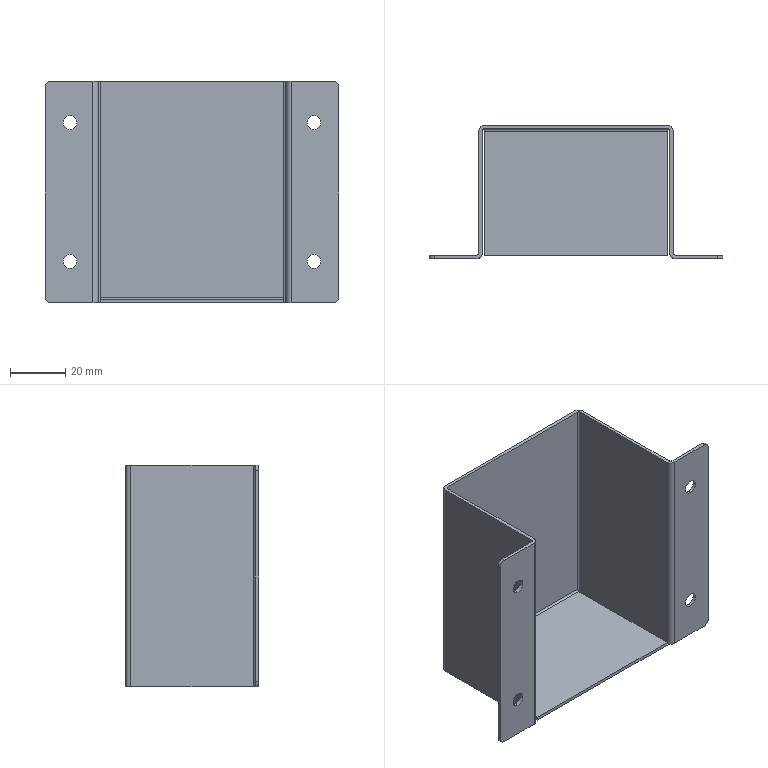Part | SolidWorks | features BaseBody 1 | 1 solid | 44 faces | box 106 x 48 x 80 mm | volume 22432 mm3 | cylinder 22 | plane 22 | commonest cylinder face diameters 5 x8 1.473 x5 3.873 x5 4 x4
STEP:
#1=CARTESIAN_POINT('',(79.,-1.2,67.5));
#2=VERTEX_POINT('',#1);
#3=CARTESIAN_POINT('',(79.,-1.2,62.5));
#4=VERTEX_POINT('',#3);
#5=CARTESIAN_POINT('',(79.,-1.2,65.));
#6=DIRECTION('',(0.,-1.,0.));
#7=DIRECTION('',(0.,0.,1.));
#8=AXIS2_PLACEMENT_3D('',#5,#6,#7);
#9=CIRCLE('',#8,2.5);
#10=EDGE_CURVE('',#2,#4,#9,.T.);
#11=ORIENTED_EDGE('',*,*,#10,.T.);
#12=CARTESIAN_POINT('',(79.,0.,62.5));
#13=VERTEX_POINT('',#12);
#14=CARTESIAN_POINT('',(79.,0.,62.5));
#15=DIRECTION('',(0.,1.,0.));
#16=VECTOR('',#15,1000.);
#17=LINE('',#14,#16);
#18=EDGE_CURVE('',#4,#13,#17,.T.);
#19=ORIENTED_EDGE('',*,*,#18,.T.);
#20=CARTESIAN_POINT('',(79.,0.,67.5));
#21=VERTEX_POINT('',#20);
#22=CARTESIAN_POINT('',(79.,0.,65.));
#23=DIRECTION('',(0.,-1.,0.));
#24=DIRECTION('',(0.,0.,1.));
#25=AXIS2_PLACEMENT_3D('',#22,#23,#24);
#26=CIRCLE('',#25,2.5);
#27=EDGE_CURVE('',#21,#13,#26,.T.);
#28=ORIENTED_EDGE('',*,*,#27,.F.);
#29=CARTESIAN_POINT('',(79.,0.,67.5));
#30=DIRECTION('',(0.,1.,0.));
#31=VECTOR('',#30,1000.);
#32=LINE('',#29,#31);
#33=EDGE_CURVE('',#2,#21,#32,.T.);
#34=ORIENTED_EDGE('',*,*,#33,.F.);
#35=EDGE_LOOP('',(#11,#19,#28,#34));
#36=FACE_OUTER_BOUND('',#35,.T.);
#37=CARTESIAN_POINT('',(79.,0.,65.));
#38=DIRECTION('',(0.,1.,0.));
#39=DIRECTION('',(0.,0.,1.));
#40=AXIS2_PLACEMENT_3D('',#37,#38,#39);
#41=CYLINDRICAL_SURFACE('',#40,2.5);
#42=ADVANCED_FACE('',(#36),#41,.F.);
#43=CARTESIAN_POINT('',(79.,-1.2,17.5));
#44=VERTEX_POINT('',#43);
#45=CARTESIAN_POINT('',(79.,-1.2,12.5));
#46=VERTEX_POINT('',#45);
#47=CARTESIAN_POINT('',(79.,-1.2,15.));
#48=DIRECTION('',(0.,-1.,0.));
#49=DIRECTION('',(0.,0.,1.));
#50=AXIS2_PLACEMENT_3D('',#47,#48,#49);
#51=CIRCLE('',#50,2.5);
#52=EDGE_CURVE('',#44,#46,#51,.T.);
#53=ORIENTED_EDGE('',*,*,#52,.T.);
#54=CARTESIAN_POINT('',(79.,0.,12.5));
#55=VERTEX_POINT('',#54);
#56=CARTESIAN_POINT('',(79.,0.,12.5));
#57=DIRECTION('',(0.,1.,0.));
#58=VECTOR('',#57,1000.);
#59=LINE('',#56,#58);
#60=EDGE_CURVE('',#46,#55,#59,.T.);
#61=ORIENTED_EDGE('',*,*,#60,.T.);
#62=CARTESIAN_POINT('',(79.,0.,17.5));
#63=VERTEX_POINT('',#62);
#64=CARTESIAN_POINT('',(79.,0.,15.));
#65=DIRECTION('',(0.,-1.,0.));
#66=DIRECTION('',(0.,0.,1.));
#67=AXIS2_PLACEMENT_3D('',#64,#65,#66);
#68=CIRCLE('',#67,2.5);
#69=EDGE_CURVE('',#63,#55,#68,.T.);
#70=ORIENTED_EDGE('',*,*,#69,.F.);
#71=CARTESIAN_POINT('',(79.,0.,17.5));
#72=DIRECTION('',(0.,1.,0.));
#73=VECTOR('',#72,1000.);
#74=LINE('',#71,#73);
#75=EDGE_CURVE('',#44,#63,#74,.T.);
#76=ORIENTED_EDGE('',*,*,#75,.F.);
#77=EDGE_LOOP('',(#53,#61,#70,#76));
#78=FACE_OUTER_BOUND('',#77,.T.);
#79=CARTESIAN_POINT('',(79.,0.,15.));
#80=DIRECTION('',(0.,1.,0.));
#81=DIRECTION('',(0.,0.,1.));
#82=AXIS2_PLACEMENT_3D('',#79,#80,#81);
#83=CYLINDRICAL_SURFACE('',#82,2.5);
#84=ADVANCED_FACE('',(#78),#83,.F.);
#85=CARTESIAN_POINT('',(-9.,-1.2,67.5));
#86=VERTEX_POINT('',#85);
#87=CARTESIAN_POINT('',(-9.,-1.2,62.5));
#88=VERTEX_POINT('',#87);
#89=CARTESIAN_POINT('',(-9.,-1.2,65.));
#90=DIRECTION('',(0.,-1.,0.));
#91=DIRECTION('',(0.,0.,1.));
#92=AXIS2_PLACEMENT_3D('',#89,#90,#91);
#93=CIRCLE('',#92,2.5);
#94=EDGE_CURVE('',#86,#88,#93,.T.);
#95=ORIENTED_EDGE('',*,*,#94,.T.);
#96=CARTESIAN_POINT('',(-9.,0.,62.5));
#97=VERTEX_POINT('',#96);
#98=CARTESIAN_POINT('',(-9.,0.,62.5));
#99=DIRECTION('',(0.,1.,0.));
#100=VECTOR('',#99,1000.);
#101=LINE('',#98,#100);
#102=EDGE_CURVE('',#88,#97,#101,.T.);
#103=ORIENTED_EDGE('',*,*,#102,.T.);
#104=CARTESIAN_POINT('',(-9.,0.,67.5));
#105=VERTEX_POINT('',#104);
#106=CARTESIAN_POINT('',(-9.,0.,65.));
#107=DIRECTION('',(0.,-1.,0.));
#108=DIRECTION('',(0.,0.,1.));
#109=AXIS2_PLACEMENT_3D('',#106,#107,#108);
#110=CIRCLE('',#109,2.5);
#111=EDGE_CURVE('',#105,#97,#110,.T.);
#112=ORIENTED_EDGE('',*,*,#111,.F.);
#113=CARTESIAN_POINT('',(-9.,0.,67.5));
#114=DIRECTION('',(0.,1.,0.));
#115=VECTOR('',#114,1000.);
#116=LINE('',#113,#115);
#117=EDGE_CURVE('',#86,#105,#116,.T.);
#118=ORIENTED_EDGE('',*,*,#117,.F.);
#119=EDGE_LOOP('',(#95,#103,#112,#118));
#120=FACE_OUTER_BOUND('',#119,.T.);
#121=CARTESIAN_POINT('',(-9.,0.,65.));
#122=DIRECTION('',(0.,1.,0.));
#123=DIRECTION('',(0.,0.,1.));
#124=AXIS2_PLACEMENT_3D('',#121,#122,#123);
#125=CYLINDRICAL_SURFACE('',#124,2.5);
#126=ADVANCED_FACE('',(#120),#125,.F.);
#127=CARTESIAN_POINT('',(-9.,-1.2,17.5));
#128=VERTEX_POINT('',#127);
#129=CARTESIAN_POINT('',(-9.,-1.2,12.5));
#130=VERTEX_POINT('',#129);
#131=CARTESIAN_POINT('',(-9.,-1.2,15.));
#132=DIRECTION('',(0.,-1.,0.));
#133=DIRECTION('',(0.,0.,1.));
#134=AXIS2_PLACEMENT_3D('',#131,#132,#133);
#135=CIRCLE('',#134,2.5);
#136=EDGE_CURVE('',#128,#130,#135,.T.);
#137=ORIENTED_EDGE('',*,*,#136,.T.);
#138=CARTESIAN_POINT('',(-9.,0.,12.5));
#139=VERTEX_POINT('',#138);
#140=CARTESIAN_POINT('',(-9.,0.,12.5));
#141=DIRECTION('',(0.,1.,0.));
#142=VECTOR('',#141,1000.);
#143=LINE('',#140,#142);
#144=EDGE_CURVE('',#130,#139,#143,.T.);
#145=ORIENTED_EDGE('',*,*,#144,.T.);
#146=CARTESIAN_POINT('',(-9.,0.,17.5));
#147=VERTEX_POINT('',#146);
#148=CARTESIAN_POINT('',(-9.,0.,15.));
#149=DIRECTION('',(0.,-1.,0.));
#150=DIRECTION('',(0.,0.,1.));
#151=AXIS2_PLACEMENT_3D('',#148,#149,#150);
#152=CIRCLE('',#151,2.5);
#153=EDGE_CURVE('',#147,#139,#152,.T.);
#154=ORIENTED_EDGE('',*,*,#153,.F.);
#155=CARTESIAN_POINT('',(-9.,0.,17.5));
#156=DIRECTION('',(0.,1.,0.));
#157=VECTOR('',#156,1000.);
#158=LINE('',#155,#157);
#159=EDGE_CURVE('',#128,#147,#158,.T.);
#160=ORIENTED_EDGE('',*,*,#159,.F.);
#161=EDGE_LOOP('',(#137,#145,#154,#160));
#162=FACE_OUTER_BOUND('',#161,.T.);
#163=CARTESIAN_POINT('',(-9.,0.,15.));
#164=DIRECTION('',(0.,1.,0.));
#165=DIRECTION('',(0.,0.,1.));
#166=AXIS2_PLACEMENT_3D('',#163,#164,#165);
#167=CYLINDRICAL_SURFACE('',#166,2.5);
#168=ADVANCED_FACE('',(#162),#167,.F.);
#169=CARTESIAN_POINT('',(68.063,45.6,80.));
#170=VERTEX_POINT('',#169);
#171=CARTESIAN_POINT('',(68.063,45.6,1.937));
#172=VERTEX_POINT('',#171);
#173=CARTESIAN_POINT('',(68.063,45.6,80.));
#174=DIRECTION('',(0.,0.,-1.));
#175=VECTOR('',#174,1000.);
#176=LINE('',#173,#175);
#177=EDGE_CURVE('',#170,#172,#176,.T.);
#178=ORIENTED_EDGE('',*,*,#177,.F.);
#179=CARTESIAN_POINT('',(1.937,45.6,80.));
#180=VERTEX_POINT('',#179);
#181=CARTESIAN_POINT('',(0.,45.6,80.));
#182=DIRECTION('',(1.,0.,0.));
#183=VECTOR('',#182,1000.);
#184=LINE('',#181,#183);
#185=EDGE_CURVE('',#180,#170,#184,.T.);
#186=ORIENTED_EDGE('',*,*,#185,.F.);
#187=CARTESIAN_POINT('',(1.937,45.6,1.937));
#188=VERTEX_POINT('',#187);
#189=CARTESIAN_POINT('',(1.937,45.6,80.));
#190=DIRECTION('',(0.,0.,1.));
#191=VECTOR('',#190,1000.);
#192=LINE('',#189,#191);
#193=EDGE_CURVE('',#188,#180,#192,.T.);
#194=ORIENTED_EDGE('',*,*,#193,.F.);
#195=CARTESIAN_POINT('',(0.,45.6,1.937));
#196=DIRECTION('',(-1.,0.,0.));
#197=VECTOR('',#196,1000.);
#198=LINE('',#195,#197);
#199=EDGE_CURVE('',#172,#188,#198,.T.);
#200=ORIENTED_EDGE('',*,*,#199,.F.);
#201=EDGE_LOOP('',(#178,#186,#194,#200));
#202=FACE_OUTER_BOUND('',#201,.T.);
#203=CARTESIAN_POINT('',(0.,45.6,80.));
#204=DIRECTION('',(0.,1.,0.));
#205=DIRECTION('',(0.,0.,1.));
#206=AXIS2_PLACEMENT_3D('',#203,#204,#205);
#207=PLANE('',#206);
#208=ADVANCED_FACE('',(#202),#207,.F.);
#209=CARTESIAN_POINT('',(1.937,44.863,1.2));
#210=VERTEX_POINT('',#209);
#211=CARTESIAN_POINT('',(1.937,44.863,1.937));
#212=DIRECTION('',(1.,0.,0.));
#213=DIRECTION('',(0.,0.,-1.));
#214=AXIS2_PLACEMENT_3D('',#211,#212,#213);
#215=CIRCLE('',#214,0.7366);
#216=EDGE_CURVE('',#210,#188,#215,.T.);
#217=ORIENTED_EDGE('',*,*,#216,.F.);
#218=CARTESIAN_POINT('',(68.063,44.863,1.2));
#219=VERTEX_POINT('',#218);
#220=CARTESIAN_POINT('',(68.063,44.863,1.2));
#221=DIRECTION('',(-1.,0.,0.));
#222=VECTOR('',#221,1000.);
#223=LINE('',#220,#222);
#224=EDGE_CURVE('',#219,#210,#223,.T.);
#225=ORIENTED_EDGE('',*,*,#224,.F.);
#226=CARTESIAN_POINT('',(68.063,44.863,1.937));
#227=DIRECTION('',(1.,0.,0.));
#228=DIRECTION('',(0.,0.,-1.));
#229=AXIS2_PLACEMENT_3D('',#226,#227,#228);
#230=CIRCLE('',#229,0.7366);
#231=EDGE_CURVE('',#219,#172,#230,.T.);
#232=ORIENTED_EDGE('',*,*,#231,.T.);
#233=ORIENTED_EDGE('',*,*,#199,.T.);
#234=EDGE_LOOP('',(#217,#225,#232,#233));
#235=FACE_OUTER_BOUND('',#234,.T.);
#236=CARTESIAN_POINT('',(68.063,44.863,1.937));
#237=DIRECTION('',(1.,0.,0.));
#238=DIRECTION('',(0.,0.,-1.));
#239=AXIS2_PLACEMENT_3D('',#236,#237,#238);
#240=CYLINDRICAL_SURFACE('',#239,0.7366);
#241=ADVANCED_FACE('',(#235),#240,.F.);
#242=CARTESIAN_POINT('',(68.8,44.863,80.));
#243=VERTEX_POINT('',#242);
#244=CARTESIAN_POINT('',(68.8,44.863,0.));
#245=VERTEX_POINT('',#244);
#246=CARTESIAN_POINT('',(68.8,44.863,80.));
#247=DIRECTION('',(0.,0.,-1.));
#248=VECTOR('',#247,1000.);
#249=LINE('',#246,#248);
#250=EDGE_CURVE('',#243,#245,#249,.T.);
#251=ORIENTED_EDGE('',*,*,#250,.F.);
#252=CARTESIAN_POINT('',(68.063,44.863,80.));
#253=DIRECTION('',(0.,0.,-1.));
#254=DIRECTION('',(-1.,0.,0.));
#255=AXIS2_PLACEMENT_3D('',#252,#253,#254);
#256=CIRCLE('',#255,0.7366);
#257=EDGE_CURVE('',#170,#243,#256,.T.);
#258=ORIENTED_EDGE('',*,*,#257,.F.);
#259=ORIENTED_EDGE('',*,*,#177,.T.);
#260=CARTESIAN_POINT('',(68.063,45.6,0.1456));
#261=VERTEX_POINT('',#260);
#262=CARTESIAN_POINT('',(68.063,45.6,80.));
#263=DIRECTION('',(0.,0.,1.));
#264=VECTOR('',#263,1000.);
#265=LINE('',#262,#264);
#266=EDGE_CURVE('',#261,#172,#265,.T.);
#267=ORIENTED_EDGE('',*,*,#266,.F.);
#268=CARTESIAN_POINT('',(68.063,45.6,0.));
#269=VERTEX_POINT('',#268);
#270=CARTESIAN_POINT('',(68.063,45.6,0.));
#271=DIRECTION('',(0.,0.,1.));
#272=VECTOR('',#271,1000.);
#273=LINE('',#270,#272);
#274=EDGE_CURVE('',#269,#261,#273,.T.);
#275=ORIENTED_EDGE('',*,*,#274,.F.);
#276=CARTESIAN_POINT('',(68.063,44.863,0.));
#277=DIRECTION('',(0.,0.,1.));
#278=DIRECTION('',(-1.,0.,0.));
#279=AXIS2_PLACEMENT_3D('',#276,#277,#278);
#280=CIRCLE('',#279,0.7366);
#281=EDGE_CURVE('',#245,#269,#280,.T.);
#282=ORIENTED_EDGE('',*,*,#281,.F.);
#283=EDGE_LOOP('',(#251,#258,#259,#267,#275,#282));
#284=FACE_OUTER_BOUND('',#283,.T.);
#285=CARTESIAN_POINT('',(68.063,44.863,80.));
#286=DIRECTION('',(0.,0.,-1.));
#287=DIRECTION('',(-1.,0.,0.));
#288=AXIS2_PLACEMENT_3D('',#285,#286,#287);
#289=CYLINDRICAL_SURFACE('',#288,0.7366);
#290=ADVANCED_FACE('',(#284),#289,.F.);
#291=ORIENTED_EDGE('',*,*,#185,.T.);
#292=ORIENTED_EDGE('',*,*,#257,.T.);
#293=CARTESIAN_POINT('',(68.8,0.7366,80.));
#294=VERTEX_POINT('',#293);
#295=CARTESIAN_POINT('',(68.8,46.8,80.));
#296=DIRECTION('',(0.,-1.,0.));
#297=VECTOR('',#296,1000.);
#298=LINE('',#295,#297);
#299=EDGE_CURVE('',#243,#294,#298,.T.);
#300=ORIENTED_EDGE('',*,*,#299,.T.);
#301=CARTESIAN_POINT('',(70.737,-1.2,80.));
#302=VERTEX_POINT('',#301);
#303=CARTESIAN_POINT('',(70.737,0.7366,80.));
#304=DIRECTION('',(0.,0.,-1.));
#305=DIRECTION('',(-1.,0.,0.));
#306=AXIS2_PLACEMENT_3D('',#303,#304,#305);
#307=CIRCLE('',#306,1.937);
#308=EDGE_CURVE('',#302,#294,#307,.T.);
#309=ORIENTED_EDGE('',*,*,#308,.F.);
#310=CARTESIAN_POINT('',(86.,-1.2,80.));
#311=VERTEX_POINT('',#310);
#312=CARTESIAN_POINT('',(70.,-1.2,80.));
#313=DIRECTION('',(1.,0.,0.));
#314=VECTOR('',#313,1000.);
#315=LINE('',#312,#314);
#316=EDGE_CURVE('',#302,#311,#315,.T.);
#317=ORIENTED_EDGE('',*,*,#316,.T.);
#318=CARTESIAN_POINT('',(86.,0.,80.));
#319=VERTEX_POINT('',#318);
#320=CARTESIAN_POINT('',(86.,0.,80.));
#321=DIRECTION('',(0.,-1.,0.));
#322=VECTOR('',#321,1000.);
#323=LINE('',#320,#322);
#324=EDGE_CURVE('',#319,#311,#323,.T.);
#325=ORIENTED_EDGE('',*,*,#324,.F.);
#326=CARTESIAN_POINT('',(70.737,0.,80.));
#327=VERTEX_POINT('',#326);
#328=CARTESIAN_POINT('',(68.8,0.,80.));
#329=DIRECTION('',(-1.,0.,0.));
#330=VECTOR('',#329,1000.);
#331=LINE('',#328,#330);
#332=EDGE_CURVE('',#319,#327,#331,.T.);
#333=ORIENTED_EDGE('',*,*,#332,.T.);
#334=CARTESIAN_POINT('',(70.,0.7366,80.));
#335=VERTEX_POINT('',#334);
#336=CARTESIAN_POINT('',(70.737,0.7366,80.));
#337=DIRECTION('',(0.,0.,-1.));
#338=DIRECTION('',(-1.,0.,0.));
#339=AXIS2_PLACEMENT_3D('',#336,#337,#338);
#340=CIRCLE('',#339,0.7366);
#341=EDGE_CURVE('',#327,#335,#340,.T.);
#342=ORIENTED_EDGE('',*,*,#341,.T.);
#343=CARTESIAN_POINT('',(70.,44.863,80.));
#344=VERTEX_POINT('',#343);
#345=CARTESIAN_POINT('',(70.,45.6,80.));
#346=DIRECTION('',(0.,1.,0.));
#347=VECTOR('',#346,1000.);
#348=LINE('',#345,#347);
#349=EDGE_CURVE('',#335,#344,#348,.T.);
#350=ORIENTED_EDGE('',*,*,#349,.T.);
#351=CARTESIAN_POINT('',(68.063,46.8,80.));
#352=VERTEX_POINT('',#351);
#353=CARTESIAN_POINT('',(68.063,44.863,80.));
#354=DIRECTION('',(0.,0.,-1.));
#355=DIRECTION('',(-1.,0.,0.));
#356=AXIS2_PLACEMENT_3D('',#353,#354,#355);
#357=CIRCLE('',#356,1.937);
#358=EDGE_CURVE('',#352,#344,#357,.T.);
#359=ORIENTED_EDGE('',*,*,#358,.F.);
#360=CARTESIAN_POINT('',(1.937,46.8,80.));
#361=VERTEX_POINT('',#360);
#362=CARTESIAN_POINT('',(1.2,46.8,80.));
#363=DIRECTION('',(-1.,0.,0.));
#364=VECTOR('',#363,1000.);
#365=LINE('',#362,#364);
#366=EDGE_CURVE('',#352,#361,#365,.T.);
#367=ORIENTED_EDGE('',*,*,#366,.T.);
#368=CARTESIAN_POINT('',(0.,44.863,80.));
#369=VERTEX_POINT('',#368);
#370=CARTESIAN_POINT('',(1.937,44.863,80.));
#371=DIRECTION('',(0.,0.,-1.));
#372=DIRECTION('',(-1.,0.,0.));
#373=AXIS2_PLACEMENT_3D('',#370,#371,#372);
#374=CIRCLE('',#373,1.937);
#375=EDGE_CURVE('',#369,#361,#374,.T.);
#376=ORIENTED_EDGE('',*,*,#375,.F.);
#377=CARTESIAN_POINT('',(0.,0.7366,80.));
#378=VERTEX_POINT('',#377);
#379=CARTESIAN_POINT('',(0.,-1.2,80.));
#380=DIRECTION('',(0.,-1.,0.));
#381=VECTOR('',#380,1000.);
#382=LINE('',#379,#381);
#383=EDGE_CURVE('',#369,#378,#382,.T.);
#384=ORIENTED_EDGE('',*,*,#383,.T.);
#385=CARTESIAN_POINT('',(-0.7366,0.,80.));
#386=VERTEX_POINT('',#385);
#387=CARTESIAN_POINT('',(-0.7366,0.7366,80.));
#388=DIRECTION('',(0.,0.,-1.));
#389=DIRECTION('',(-1.,0.,0.));
#390=AXIS2_PLACEMENT_3D('',#387,#388,#389);
#391=CIRCLE('',#390,0.7366);
#392=EDGE_CURVE('',#378,#386,#391,.T.);
#393=ORIENTED_EDGE('',*,*,#392,.T.);
#394=CARTESIAN_POINT('',(-16.,0.,80.));
#395=VERTEX_POINT('',#394);
#396=CARTESIAN_POINT('',(70.737,0.,80.));
#397=DIRECTION('',(1.,0.,0.));
#398=VECTOR('',#397,1000.);
#399=LINE('',#396,#398);
#400=EDGE_CURVE('',#395,#386,#399,.T.);
#401=ORIENTED_EDGE('',*,*,#400,.F.);
#402=CARTESIAN_POINT('',(-16.,-1.2,80.));
#403=VERTEX_POINT('',#402);
#404=CARTESIAN_POINT('',(-16.,0.7366,80.));
#405=DIRECTION('',(0.,1.,0.));
#406=VECTOR('',#405,1000.);
#407=LINE('',#404,#406);
#408=EDGE_CURVE('',#403,#395,#407,.T.);
#409=ORIENTED_EDGE('',*,*,#408,.F.);
#410=CARTESIAN_POINT('',(-0.7366,-1.2,80.));
#411=VERTEX_POINT('',#410);
#412=CARTESIAN_POINT('',(0.,-1.2,80.));
#413=DIRECTION('',(1.,0.,0.));
#414=VECTOR('',#413,1000.);
#415=LINE('',#412,#414);
#416=EDGE_CURVE('',#403,#411,#415,.T.);
#417=ORIENTED_EDGE('',*,*,#416,.T.);
#418=CARTESIAN_POINT('',(1.2,0.7366,80.));
#419=VERTEX_POINT('',#418);
#420=CARTESIAN_POINT('',(-0.7366,0.7366,80.));
#421=DIRECTION('',(0.,0.,-1.));
#422=DIRECTION('',(-1.,0.,0.));
#423=AXIS2_PLACEMENT_3D('',#420,#421,#422);
#424=CIRCLE('',#423,1.937);
#425=EDGE_CURVE('',#419,#411,#424,.T.);
#426=ORIENTED_EDGE('',*,*,#425,.F.);
#427=CARTESIAN_POINT('',(1.2,44.863,80.));
#428=VERTEX_POINT('',#427);
#429=CARTESIAN_POINT('',(1.2,46.8,80.));
#430=DIRECTION('',(0.,1.,0.));
#431=VECTOR('',#430,1000.);
#432=LINE('',#429,#431);
#433=EDGE_CURVE('',#419,#428,#432,.T.);
#434=ORIENTED_EDGE('',*,*,#433,.T.);
#435=CARTESIAN_POINT('',(1.937,44.863,80.));
#436=DIRECTION('',(0.,0.,-1.));
#437=DIRECTION('',(-1.,0.,0.));
#438=AXIS2_PLACEMENT_3D('',#435,#436,#437);
#439=CIRCLE('',#438,0.7366);
#440=EDGE_CURVE('',#428,#180,#439,.T.);
#441=ORIENTED_EDGE('',*,*,#440,.T.);
#442=EDGE_LOOP('',(#291,#292,#300,#309,#317,#325,#333,#342,#350,#359,#367,#376,#384,#393,#401,#409,#417,#426,#434,#441));
#443=FACE_OUTER_BOUND('',#442,.T.);
#444=CARTESIAN_POINT('',(1.2,44.863,80.));
#445=DIRECTION('',(0.,0.,1.));
#446=DIRECTION('',(1.,0.,0.));
#447=AXIS2_PLACEMENT_3D('',#444,#445,#446);
#448=PLANE('',#447);
#449=ADVANCED_FACE('',(#443),#448,.T.);
#450=CARTESIAN_POINT('',(1.937,45.6,0.1456));
#451=VERTEX_POINT('',#450);
#452=CARTESIAN_POINT('',(1.937,45.6,0.));
#453=VERTEX_POINT('',#452);
#454=CARTESIAN_POINT('',(1.937,45.6,1.937));
#455=DIRECTION('',(0.,0.,-1.));
#456=VECTOR('',#455,1000.);
#457=LINE('',#454,#456);
#458=EDGE_CURVE('',#451,#453,#457,.T.);
#459=ORIENTED_EDGE('',*,*,#458,.F.);
#460=CARTESIAN_POINT('',(1.937,45.6,80.));
#461=DIRECTION('',(0.,0.,-1.));
#462=VECTOR('',#461,1000.);
#463=LINE('',#460,#462);
#464=EDGE_CURVE('',#188,#451,#463,.T.);
#465=ORIENTED_EDGE('',*,*,#464,.F.);
#466=ORIENTED_EDGE('',*,*,#193,.T.);
#467=ORIENTED_EDGE('',*,*,#440,.F.);
#468=CARTESIAN_POINT('',(1.2,44.863,0.));
#469=VERTEX_POINT('',#468);
#470=CARTESIAN_POINT('',(1.2,44.863,80.));
#471=DIRECTION('',(0.,0.,1.));
#472=VECTOR('',#471,1000.);
#473=LINE('',#470,#472);
#474=EDGE_CURVE('',#469,#428,#473,.T.);
#475=ORIENTED_EDGE('',*,*,#474,.F.);
#476=CARTESIAN_POINT('',(1.937,44.863,0.));
#477=DIRECTION('',(0.,0.,1.));
#478=DIRECTION('',(-1.,0.,0.));
#479=AXIS2_PLACEMENT_3D('',#476,#477,#478);
#480=CIRCLE('',#479,0.7366);
#481=EDGE_CURVE('',#453,#469,#480,.T.);
#482=ORIENTED_EDGE('',*,*,#481,.F.);
#483=EDGE_LOOP('',(#459,#465,#466,#467,#475,#482));
#484=FACE_OUTER_BOUND('',#483,.T.);
#485=CARTESIAN_POINT('',(1.937,44.863,80.));
#486=DIRECTION('',(0.,0.,-1.));
#487=DIRECTION('',(-1.,0.,0.));
#488=AXIS2_PLACEMENT_3D('',#485,#486,#487);
#489=CYLINDRICAL_SURFACE('',#488,0.7366);
#490=ADVANCED_FACE('',(#484),#489,.F.);
#491=CARTESIAN_POINT('',(1.937,-0.2,1.2));
#492=VERTEX_POINT('',#491);
#493=CARTESIAN_POINT('',(1.937,0.,1.2));
#494=DIRECTION('',(0.,1.,0.));
#495=VECTOR('',#494,1000.);
#496=LINE('',#493,#495);
#497=EDGE_CURVE('',#492,#210,#496,.T.);
#498=ORIENTED_EDGE('',*,*,#497,.F.);
#499=CARTESIAN_POINT('',(68.063,-0.2,1.2));
#500=VERTEX_POINT('',#499);
#501=CARTESIAN_POINT('',(0.,-0.2,1.2));
#502=DIRECTION('',(-1.,0.,0.));
#503=VECTOR('',#502,1000.);
#504=LINE('',#501,#503);
#505=EDGE_CURVE('',#500,#492,#504,.T.);
#506=ORIENTED_EDGE('',*,*,#505,.F.);
#507=CARTESIAN_POINT('',(68.063,0.,1.2));
#508=DIRECTION('',(0.,-1.,0.));
#509=VECTOR('',#508,1000.);
#510=LINE('',#507,#509);
#511=EDGE_CURVE('',#219,#500,#510,.T.);
#512=ORIENTED_EDGE('',*,*,#511,.F.);
#513=ORIENTED_EDGE('',*,*,#224,.T.);
#514=EDGE_LOOP('',(#498,#506,#512,#513));
#515=FACE_OUTER_BOUND('',#514,.T.);
#516=CARTESIAN_POINT('',(0.,0.,1.2));
#517=DIRECTION('',(0.,0.,-1.));
#518=DIRECTION('',(0.,1.,0.));
#519=AXIS2_PLACEMENT_3D('',#516,#517,#518);
#520=PLANE('',#519);
#521=ADVANCED_FACE('',(#515),#520,.F.);
#522=CARTESIAN_POINT('',(68.8,0.7366,0.));
#523=VERTEX_POINT('',#522);
#524=CARTESIAN_POINT('',(68.8,0.7366,80.));
#525=DIRECTION('',(0.,0.,-1.));
#526=VECTOR('',#525,1000.);
#527=LINE('',#524,#526);
#528=EDGE_CURVE('',#294,#523,#527,.T.);
#529=ORIENTED_EDGE('',*,*,#528,.F.);
#530=ORIENTED_EDGE('',*,*,#299,.F.);
#531=ORIENTED_EDGE('',*,*,#250,.T.);
#532=CARTESIAN_POINT('',(68.8,46.8,0.));
#533=DIRECTION('',(0.,1.,0.));
#534=VECTOR('',#533,1000.);
#535=LINE('',#532,#534);
#536=EDGE_CURVE('',#523,#245,#535,.T.);
#537=ORIENTED_EDGE('',*,*,#536,.F.);
#538=EDGE_LOOP('',(#529,#530,#531,#537));
#539=FACE_OUTER_BOUND('',#538,.T.);
#540=CARTESIAN_POINT('',(68.8,46.8,80.));
#541=DIRECTION('',(1.,0.,0.));
#542=DIRECTION('',(0.,0.,-1.));
#543=AXIS2_PLACEMENT_3D('',#540,#541,#542);
#544=PLANE('',#543);
#545=ADVANCED_FACE('',(#539),#544,.F.);
#546=ORIENTED_EDGE('',*,*,#266,.T.);
#547=ORIENTED_EDGE('',*,*,#231,.F.);
#548=ORIENTED_EDGE('',*,*,#511,.T.);
#549=CARTESIAN_POINT('',(68.063,-0.2,0.));
#550=VERTEX_POINT('',#549);
#551=CARTESIAN_POINT('',(68.063,-0.2,0.));
#552=DIRECTION('',(0.,0.,1.));
#553=VECTOR('',#552,1000.);
#554=LINE('',#551,#553);
#555=EDGE_CURVE('',#550,#500,#554,.T.);
#556=ORIENTED_EDGE('',*,*,#555,.F.);
#557=CARTESIAN_POINT('',(68.063,44.863,0.));
#558=VERTEX_POINT('',#557);
#559=CARTESIAN_POINT('',(68.063,45.6,0.));
#560=DIRECTION('',(0.,1.,0.));
#561=VECTOR('',#560,1000.);
#562=LINE('',#559,#561);
#563=EDGE_CURVE('',#550,#558,#562,.T.);
#564=ORIENTED_EDGE('',*,*,#563,.T.);
#565=CARTESIAN_POINT('',(68.063,44.863,1.937));
#566=DIRECTION('',(-1.,0.,0.));
#567=DIRECTION('',(0.,0.,-1.));
#568=AXIS2_PLACEMENT_3D('',#565,#566,#567);
#569=CIRCLE('',#568,1.937);
#570=EDGE_CURVE('',#261,#558,#569,.T.);
#571=ORIENTED_EDGE('',*,*,#570,.F.);
#572=EDGE_LOOP('',(#546,#547,#548,#556,#564,#571));
#573=FACE_OUTER_BOUND('',#572,.T.);
#574=CARTESIAN_POINT('',(68.063,44.863,1.937));
#575=DIRECTION('',(-1.,0.,0.));
#576=DIRECTION('',(0.,0.,1.));
#577=AXIS2_PLACEMENT_3D('',#574,#575,#576);
#578=PLANE('',#577);
#579=ADVANCED_FACE('',(#573),#578,.F.);
#580=CARTESIAN_POINT('',(1.937,46.8,1.937));
#581=VERTEX_POINT('',#580);
#582=CARTESIAN_POINT('',(1.937,46.8,80.));
#583=DIRECTION('',(0.,0.,1.));
#584=VECTOR('',#583,1000.);
#585=LINE('',#582,#584);
#586=EDGE_CURVE('',#581,#361,#585,.T.);
#587=ORIENTED_EDGE('',*,*,#586,.T.);
#588=ORIENTED_EDGE('',*,*,#366,.F.);
#589=CARTESIAN_POINT('',(68.063,46.8,1.937));
#590=VERTEX_POINT('',#589);
#591=CARTESIAN_POINT('',(68.063,46.8,80.));
#592=DIRECTION('',(0.,0.,-1.));
#593=VECTOR('',#592,1000.);
#594=LINE('',#591,#593);
#595=EDGE_CURVE('',#352,#590,#594,.T.);
#596=ORIENTED_EDGE('',*,*,#595,.T.);
#597=CARTESIAN_POINT('',(0.,46.8,1.937));
#598=DIRECTION('',(-1.,0.,0.));
#599=VECTOR('',#598,1000.);
#600=LINE('',#597,#599);
#601=EDGE_CURVE('',#590,#581,#600,.T.);
#602=ORIENTED_EDGE('',*,*,#601,.T.);
#603=EDGE_LOOP('',(#587,#588,#596,#602));
#604=FACE_OUTER_BOUND('',#603,.T.);
#605=CARTESIAN_POINT('',(0.,46.8,80.));
#606=DIRECTION('',(0.,1.,0.));
#607=DIRECTION('',(0.,0.,1.));
#608=AXIS2_PLACEMENT_3D('',#605,#606,#607);
#609=PLANE('',#608);
#610=ADVANCED_FACE('',(#604),#609,.T.);
#611=CARTESIAN_POINT('',(1.937,44.863,0.));
#612=VERTEX_POINT('',#611);
#613=CARTESIAN_POINT('',(1.937,44.863,1.937));
#614=DIRECTION('',(-1.,0.,0.));
#615=DIRECTION('',(0.,0.,-1.));
#616=AXIS2_PLACEMENT_3D('',#613,#614,#615);
#617=CIRCLE('',#616,1.937);
#618=EDGE_CURVE('',#451,#612,#617,.T.);
#619=ORIENTED_EDGE('',*,*,#618,.T.);
#620=CARTESIAN_POINT('',(1.937,-0.2,0.));
#621=VERTEX_POINT('',#620);
#622=CARTESIAN_POINT('',(1.937,-0.2,0.));
#623=DIRECTION('',(0.,-1.,0.));
#624=VECTOR('',#623,1000.);
#625=LINE('',#622,#624);
#626=EDGE_CURVE('',#612,#621,#625,.T.);
#627=ORIENTED_EDGE('',*,*,#626,.T.);
#628=CARTESIAN_POINT('',(1.937,-0.2,0.));
#629=DIRECTION('',(0.,0.,1.));
#630=VECTOR('',#629,1000.);
#631=LINE('',#628,#630);
#632=EDGE_CURVE('',#621,#492,#631,.T.);
#633=ORIENTED_EDGE('',*,*,#632,.T.);
#634=ORIENTED_EDGE('',*,*,#497,.T.);
#635=ORIENTED_EDGE('',*,*,#216,.T.);
#636=ORIENTED_EDGE('',*,*,#464,.T.);
#637=EDGE_LOOP('',(#619,#627,#633,#634,#635,#636));
#638=FACE_OUTER_BOUND('',#637,.T.);
#639=CARTESIAN_POINT('',(1.937,44.863,1.937));
#640=DIRECTION('',(-1.,0.,0.));
#641=DIRECTION('',(0.,0.,1.));
#642=AXIS2_PLACEMENT_3D('',#639,#640,#641);
#643=PLANE('',#642);
#644=ADVANCED_FACE('',(#638),#643,.T.);
#645=ORIENTED_EDGE('',*,*,#474,.T.);
#646=ORIENTED_EDGE('',*,*,#433,.F.);
#647=CARTESIAN_POINT('',(1.2,0.7366,0.));
#648=VERTEX_POINT('',#647);
#649=CARTESIAN_POINT('',(1.2,0.7366,80.));
#650=DIRECTION('',(0.,0.,1.));
#651=VECTOR('',#650,1000.);
#652=LINE('',#649,#651);
#653=EDGE_CURVE('',#648,#419,#652,.T.);
#654=ORIENTED_EDGE('',*,*,#653,.F.);
#655=CARTESIAN_POINT('',(1.2,46.8,0.));
#656=DIRECTION('',(0.,-1.,0.));
#657=VECTOR('',#656,1000.);
#658=LINE('',#655,#657);
#659=EDGE_CURVE('',#469,#648,#658,.T.);
#660=ORIENTED_EDGE('',*,*,#659,.F.);
#661=EDGE_LOOP('',(#645,#646,#654,#660));
#662=FACE_OUTER_BOUND('',#661,.T.);
#663=CARTESIAN_POINT('',(1.2,46.8,80.));
#664=DIRECTION('',(-1.,0.,0.));
#665=DIRECTION('',(0.,-1.,0.));
#666=AXIS2_PLACEMENT_3D('',#663,#664,#665);
#667=PLANE('',#666);
#668=ADVANCED_FACE('',(#662),#667,.F.);
#669=CARTESIAN_POINT('',(68.063,-0.2,0.));
#670=DIRECTION('',(1.,0.,0.));
#671=VECTOR('',#670,1000.);
#672=LINE('',#669,#671);
#673=EDGE_CURVE('',#621,#550,#672,.T.);
#674=ORIENTED_EDGE('',*,*,#673,.T.);
#675=ORIENTED_EDGE('',*,*,#555,.T.);
#676=ORIENTED_EDGE('',*,*,#505,.T.);
#677=ORIENTED_EDGE('',*,*,#632,.F.);
#678=EDGE_LOOP('',(#674,#675,#676,#677));
#679=FACE_OUTER_BOUND('',#678,.T.);
#680=CARTESIAN_POINT('',(68.063,-0.2,0.));
#681=DIRECTION('',(0.,-1.,0.));
#682=DIRECTION('',(0.,0.,-1.));
#683=AXIS2_PLACEMENT_3D('',#680,#681,#682);
#684=PLANE('',#683);
#685=ADVANCED_FACE('',(#679),#684,.T.);
#686=ORIENTED_EDGE('',*,*,#536,.T.);
#687=ORIENTED_EDGE('',*,*,#281,.T.);
#688=CARTESIAN_POINT('',(68.063,46.8,0.));
#689=VERTEX_POINT('',#688);
#690=CARTESIAN_POINT('',(68.063,45.6,0.));
#691=DIRECTION('',(0.,-1.,0.));
#692=VECTOR('',#691,1000.);
#693=LINE('',#690,#692);
#694=EDGE_CURVE('',#689,#269,#693,.T.);
#695=ORIENTED_EDGE('',*,*,#694,.F.);
#696=CARTESIAN_POINT('',(70.,44.863,0.));
#697=VERTEX_POINT('',#696);
#698=CARTESIAN_POINT('',(68.063,44.863,0.));
#699=DIRECTION('',(0.,0.,1.));
#700=DIRECTION('',(-1.,0.,0.));
#701=AXIS2_PLACEMENT_3D('',#698,#699,#700);
#702=CIRCLE('',#701,1.937);
#703=EDGE_CURVE('',#697,#689,#702,.T.);
#704=ORIENTED_EDGE('',*,*,#703,.F.);
#705=CARTESIAN_POINT('',(70.,0.7366,0.));
#706=VERTEX_POINT('',#705);
#707=CARTESIAN_POINT('',(70.,-1.2,0.));
#708=DIRECTION('',(0.,-1.,0.));
#709=VECTOR('',#708,1000.);
#710=LINE('',#707,#709);
#711=EDGE_CURVE('',#697,#706,#710,.T.);
#712=ORIENTED_EDGE('',*,*,#711,.T.);
#713=CARTESIAN_POINT('',(70.737,0.,0.));
#714=VERTEX_POINT('',#713);
#715=CARTESIAN_POINT('',(70.737,0.7366,0.));
#716=DIRECTION('',(0.,0.,1.));
#717=DIRECTION('',(-1.,0.,0.));
#718=AXIS2_PLACEMENT_3D('',#715,#716,#717);
#719=CIRCLE('',#718,0.7366);
#720=EDGE_CURVE('',#706,#714,#719,.T.);
#721=ORIENTED_EDGE('',*,*,#720,.T.);
#722=CARTESIAN_POINT('',(86.,0.,0.));
#723=VERTEX_POINT('',#722);
#724=CARTESIAN_POINT('',(70.737,0.,0.));
#725=DIRECTION('',(1.,0.,0.));
#726=VECTOR('',#725,1000.);
#727=LINE('',#724,#726);
#728=EDGE_CURVE('',#714,#723,#727,.T.);
#729=ORIENTED_EDGE('',*,*,#728,.T.);
#730=CARTESIAN_POINT('',(86.,-1.2,0.));
#731=VERTEX_POINT('',#730);
#732=CARTESIAN_POINT('',(86.,0.7366,0.));
#733=DIRECTION('',(0.,-1.,0.));
#734=VECTOR('',#733,1000.);
#735=LINE('',#732,#734);
#736=EDGE_CURVE('',#723,#731,#735,.T.);
#737=ORIENTED_EDGE('',*,*,#736,.T.);
#738=CARTESIAN_POINT('',(70.737,-1.2,0.));
#739=VERTEX_POINT('',#738);
#740=CARTESIAN_POINT('',(70.,-1.2,0.));
#741=DIRECTION('',(-1.,0.,0.));
#742=VECTOR('',#741,1000.);
#743=LINE('',#740,#742);
#744=EDGE_CURVE('',#731,#739,#743,.T.);
#745=ORIENTED_EDGE('',*,*,#744,.T.);
#746=CARTESIAN_POINT('',(70.737,0.7366,0.));
#747=DIRECTION('',(0.,0.,1.));
#748=DIRECTION('',(-1.,0.,0.));
#749=AXIS2_PLACEMENT_3D('',#746,#747,#748);
#750=CIRCLE('',#749,1.937);
#751=EDGE_CURVE('',#523,#739,#750,.T.);
#752=ORIENTED_EDGE('',*,*,#751,.F.);
#753=EDGE_LOOP('',(#686,#687,#695,#704,#712,#721,#729,#737,#745,#752));
#754=FACE_OUTER_BOUND('',#753,.T.);
#755=CARTESIAN_POINT('',(70.737,-1.2,0.));
#756=DIRECTION('',(0.,0.,-1.));
#757=DIRECTION('',(-1.,0.,0.));
#758=AXIS2_PLACEMENT_3D('',#755,#756,#757);
#759=PLANE('',#758);
#760=ADVANCED_FACE('',(#754),#759,.T.);
#761=ORIENTED_EDGE('',*,*,#308,.T.);
#762=ORIENTED_EDGE('',*,*,#528,.T.);
#763=ORIENTED_EDGE('',*,*,#751,.T.);
#764=CARTESIAN_POINT('',(70.737,-1.2,80.));
#765=DIRECTION('',(0.,0.,1.));
#766=VECTOR('',#765,1000.);
#767=LINE('',#764,#766);
#768=EDGE_CURVE('',#739,#302,#767,.T.);
#769=ORIENTED_EDGE('',*,*,#768,.T.);
#770=EDGE_LOOP('',(#761,#762,#763,#769));
#771=FACE_OUTER_BOUND('',#770,.T.);
#772=CARTESIAN_POINT('',(70.737,0.7366,80.));
#773=DIRECTION('',(0.,0.,-1.));
#774=DIRECTION('',(-1.,0.,0.));
#775=AXIS2_PLACEMENT_3D('',#772,#773,#774);
#776=CYLINDRICAL_SURFACE('',#775,1.937);
#777=ADVANCED_FACE('',(#771),#776,.T.);
#778=ORIENTED_EDGE('',*,*,#586,.F.);
#779=CARTESIAN_POINT('',(1.937,46.8,0.));
#780=VERTEX_POINT('',#779);
#781=CARTESIAN_POINT('',(1.937,46.8,80.));
#782=DIRECTION('',(0.,0.,-1.));
#783=VECTOR('',#782,1000.);
#784=LINE('',#781,#783);
#785=EDGE_CURVE('',#581,#780,#784,.T.);
#786=ORIENTED_EDGE('',*,*,#785,.T.);
#787=CARTESIAN_POINT('',(0.,44.863,0.));
#788=VERTEX_POINT('',#787);
#789=CARTESIAN_POINT('',(1.937,44.863,0.));
#790=DIRECTION('',(0.,0.,1.));
#791=DIRECTION('',(-1.,0.,0.));
#792=AXIS2_PLACEMENT_3D('',#789,#790,#791);
#793=CIRCLE('',#792,1.937);
#794=EDGE_CURVE('',#780,#788,#793,.T.);
#795=ORIENTED_EDGE('',*,*,#794,.T.);
#796=CARTESIAN_POINT('',(0.,44.863,80.));
#797=DIRECTION('',(0.,0.,1.));
#798=VECTOR('',#797,1000.);
#799=LINE('',#796,#798);
#800=EDGE_CURVE('',#788,#369,#799,.T.);
#801=ORIENTED_EDGE('',*,*,#800,.T.);
#802=ORIENTED_EDGE('',*,*,#375,.T.);
#803=EDGE_LOOP('',(#778,#786,#795,#801,#802));
#804=FACE_OUTER_BOUND('',#803,.T.);
#805=CARTESIAN_POINT('',(1.937,44.863,80.));
#806=DIRECTION('',(0.,0.,-1.));
#807=DIRECTION('',(-1.,0.,0.));
#808=AXIS2_PLACEMENT_3D('',#805,#806,#807);
#809=CYLINDRICAL_SURFACE('',#808,1.937);
#810=ADVANCED_FACE('',(#804),#809,.T.);
#811=ORIENTED_EDGE('',*,*,#618,.F.);
#812=CARTESIAN_POINT('',(1.937,44.863,1.937));
#813=DIRECTION('',(1.,0.,0.));
#814=DIRECTION('',(0.,0.,-1.));
#815=AXIS2_PLACEMENT_3D('',#812,#813,#814);
#816=CIRCLE('',#815,1.937);
#817=EDGE_CURVE('',#451,#581,#816,.T.);
#818=ORIENTED_EDGE('',*,*,#817,.T.);
#819=ORIENTED_EDGE('',*,*,#601,.F.);
#820=CARTESIAN_POINT('',(68.063,44.863,1.937));
#821=DIRECTION('',(-1.,0.,0.));
#822=DIRECTION('',(0.,0.,-1.));
#823=AXIS2_PLACEMENT_3D('',#820,#821,#822);
#824=CIRCLE('',#823,1.937);
#825=EDGE_CURVE('',#590,#261,#824,.T.);
#826=ORIENTED_EDGE('',*,*,#825,.T.);
#827=ORIENTED_EDGE('',*,*,#570,.T.);
#828=CARTESIAN_POINT('',(68.063,44.863,0.));
#829=DIRECTION('',(-1.,0.,0.));
#830=VECTOR('',#829,1000.);
#831=LINE('',#828,#830);
#832=EDGE_CURVE('',#558,#612,#831,.T.);
#833=ORIENTED_EDGE('',*,*,#832,.T.);
#834=EDGE_LOOP('',(#811,#818,#819,#826,#827,#833));
#835=FACE_OUTER_BOUND('',#834,.T.);
#836=CARTESIAN_POINT('',(68.063,44.863,1.937));
#837=DIRECTION('',(1.,0.,0.));
#838=DIRECTION('',(0.,0.,-1.));
#839=AXIS2_PLACEMENT_3D('',#836,#837,#838);
#840=CYLINDRICAL_SURFACE('',#839,1.937);
#841=ADVANCED_FACE('',(#835),#840,.T.);
#842=ORIENTED_EDGE('',*,*,#358,.T.);
#843=CARTESIAN_POINT('',(70.,44.863,80.));
#844=DIRECTION('',(0.,0.,-1.));
#845=VECTOR('',#844,1000.);
#846=LINE('',#843,#845);
#847=EDGE_CURVE('',#344,#697,#846,.T.);
#848=ORIENTED_EDGE('',*,*,#847,.T.);
#849=ORIENTED_EDGE('',*,*,#703,.T.);
#850=CARTESIAN_POINT('',(68.063,46.8,80.));
#851=DIRECTION('',(0.,0.,1.));
#852=VECTOR('',#851,1000.);
#853=LINE('',#850,#852);
#854=EDGE_CURVE('',#689,#590,#853,.T.);
#855=ORIENTED_EDGE('',*,*,#854,.T.);
#856=ORIENTED_EDGE('',*,*,#595,.F.);
#857=EDGE_LOOP('',(#842,#848,#849,#855,#856));
#858=FACE_OUTER_BOUND('',#857,.T.);
#859=CARTESIAN_POINT('',(68.063,44.863,80.));
#860=DIRECTION('',(0.,0.,-1.));
#861=DIRECTION('',(-1.,0.,0.));
#862=AXIS2_PLACEMENT_3D('',#859,#860,#861);
#863=CYLINDRICAL_SURFACE('',#862,1.937);
#864=ADVANCED_FACE('',(#858),#863,.T.);
#865=ORIENTED_EDGE('',*,*,#659,.T.);
#866=CARTESIAN_POINT('',(-0.7366,-1.2,0.));
#867=VERTEX_POINT('',#866);
#868=CARTESIAN_POINT('',(-0.7366,0.7366,0.));
#869=DIRECTION('',(0.,0.,1.));
#870=DIRECTION('',(-1.,0.,0.));
#871=AXIS2_PLACEMENT_3D('',#868,#869,#870);
#872=CIRCLE('',#871,1.937);
#873=EDGE_CURVE('',#867,#648,#872,.T.);
#874=ORIENTED_EDGE('',*,*,#873,.F.);
#875=CARTESIAN_POINT('',(-16.,-1.2,0.));
#876=VERTEX_POINT('',#875);
#877=CARTESIAN_POINT('',(0.,-1.2,0.));
#878=DIRECTION('',(-1.,0.,0.));
#879=VECTOR('',#878,1000.);
#880=LINE('',#877,#879);
#881=EDGE_CURVE('',#867,#876,#880,.T.);
#882=ORIENTED_EDGE('',*,*,#881,.T.);
#883=CARTESIAN_POINT('',(-16.,0.,0.));
#884=VERTEX_POINT('',#883);
#885=CARTESIAN_POINT('',(-16.,0.7366,0.));
#886=DIRECTION('',(0.,-1.,0.));
#887=VECTOR('',#886,1000.);
#888=LINE('',#885,#887);
#889=EDGE_CURVE('',#884,#876,#888,.T.);
#890=ORIENTED_EDGE('',*,*,#889,.F.);
#891=CARTESIAN_POINT('',(-0.7366,0.,0.));
#892=VERTEX_POINT('',#891);
#893=CARTESIAN_POINT('',(1.2,0.,0.));
#894=DIRECTION('',(1.,0.,0.));
#895=VECTOR('',#894,1000.);
#896=LINE('',#893,#895);
#897=EDGE_CURVE('',#884,#892,#896,.T.);
#898=ORIENTED_EDGE('',*,*,#897,.T.);
#899=CARTESIAN_POINT('',(0.,0.7366,0.));
#900=VERTEX_POINT('',#899);
#901=CARTESIAN_POINT('',(-0.7366,0.7366,0.));
#902=DIRECTION('',(0.,0.,1.));
#903=DIRECTION('',(-1.,0.,0.));
#904=AXIS2_PLACEMENT_3D('',#901,#902,#903);
#905=CIRCLE('',#904,0.7366);
#906=EDGE_CURVE('',#892,#900,#905,.T.);
#907=ORIENTED_EDGE('',*,*,#906,.T.);
#908=CARTESIAN_POINT('',(0.,45.6,0.));
#909=DIRECTION('',(0.,1.,0.));
#910=VECTOR('',#909,1000.);
#911=LINE('',#908,#910);
#912=EDGE_CURVE('',#900,#788,#911,.T.);
#913=ORIENTED_EDGE('',*,*,#912,.T.);
#914=ORIENTED_EDGE('',*,*,#794,.F.);
#915=CARTESIAN_POINT('',(1.937,45.6,0.));
#916=DIRECTION('',(0.,1.,0.));
#917=VECTOR('',#916,1000.);
#918=LINE('',#915,#917);
#919=EDGE_CURVE('',#453,#780,#918,.T.);
#920=ORIENTED_EDGE('',*,*,#919,.F.);
#921=ORIENTED_EDGE('',*,*,#481,.T.);
#922=EDGE_LOOP('',(#865,#874,#882,#890,#898,#907,#913,#914,#920,#921));
#923=FACE_OUTER_BOUND('',#922,.T.);
#924=CARTESIAN_POINT('',(1.937,45.6,0.));
#925=DIRECTION('',(0.,0.,-1.));
#926=DIRECTION('',(-1.,0.,0.));
#927=AXIS2_PLACEMENT_3D('',#924,#925,#926);
#928=PLANE('',#927);
#929=ADVANCED_FACE('',(#923),#928,.T.);
#930=ORIENTED_EDGE('',*,*,#425,.T.);
#931=CARTESIAN_POINT('',(-0.7366,-1.2,80.));
#932=DIRECTION('',(0.,0.,-1.));
#933=VECTOR('',#932,1000.);
#934=LINE('',#931,#933);
#935=EDGE_CURVE('',#411,#867,#934,.T.);
#936=ORIENTED_EDGE('',*,*,#935,.T.);
#937=ORIENTED_EDGE('',*,*,#873,.T.);
#938=ORIENTED_EDGE('',*,*,#653,.T.);
#939=EDGE_LOOP('',(#930,#936,#937,#938));
#940=FACE_OUTER_BOUND('',#939,.T.);
#941=CARTESIAN_POINT('',(-0.7366,0.7366,80.));
#942=DIRECTION('',(0.,0.,-1.));
#943=DIRECTION('',(-1.,0.,0.));
#944=AXIS2_PLACEMENT_3D('',#941,#942,#943);
#945=CYLINDRICAL_SURFACE('',#944,1.937);
#946=ADVANCED_FACE('',(#940),#945,.T.);
#947=ORIENTED_EDGE('',*,*,#563,.F.);
#948=ORIENTED_EDGE('',*,*,#673,.F.);
#949=ORIENTED_EDGE('',*,*,#626,.F.);
#950=ORIENTED_EDGE('',*,*,#832,.F.);
#951=EDGE_LOOP('',(#947,#948,#949,#950));
#952=FACE_OUTER_BOUND('',#951,.T.);
#953=CARTESIAN_POINT('',(0.,0.,0.));
#954=DIRECTION('',(0.,0.,-1.));
#955=DIRECTION('',(0.,1.,0.));
#956=AXIS2_PLACEMENT_3D('',#953,#954,#955);
#957=PLANE('',#956);
#958=ADVANCED_FACE('',(#952),#957,.T.);
#959=ORIENTED_EDGE('',*,*,#349,.F.);
#960=CARTESIAN_POINT('',(70.,0.7366,80.));
#961=DIRECTION('',(0.,0.,-1.));
#962=VECTOR('',#961,1000.);
#963=LINE('',#960,#962);
#964=EDGE_CURVE('',#335,#706,#963,.T.);
#965=ORIENTED_EDGE('',*,*,#964,.T.);
#966=ORIENTED_EDGE('',*,*,#711,.F.);
#967=ORIENTED_EDGE('',*,*,#847,.F.);
#968=EDGE_LOOP('',(#959,#965,#966,#967));
#969=FACE_OUTER_BOUND('',#968,.T.);
#970=CARTESIAN_POINT('',(70.,46.8,80.));
#971=DIRECTION('',(1.,0.,0.));
#972=DIRECTION('',(0.,0.,-1.));
#973=AXIS2_PLACEMENT_3D('',#970,#971,#972);
#974=PLANE('',#973);
#975=ADVANCED_FACE('',(#969),#974,.T.);
#976=CARTESIAN_POINT('',(88.,-1.2,78.));
#977=VERTEX_POINT('',#976);
#978=CARTESIAN_POINT('',(86.,-1.2,78.));
#979=DIRECTION('',(0.,1.,0.));
#980=DIRECTION('',(0.,0.,-1.));
#981=AXIS2_PLACEMENT_3D('',#978,#979,#980);
#982=CIRCLE('',#981,2.);
#983=EDGE_CURVE('',#311,#977,#982,.T.);
#984=ORIENTED_EDGE('',*,*,#983,.F.);
#985=ORIENTED_EDGE('',*,*,#316,.F.);
#986=ORIENTED_EDGE('',*,*,#768,.F.);
#987=ORIENTED_EDGE('',*,*,#744,.F.);
#988=CARTESIAN_POINT('',(88.,-1.2,2.));
#989=VERTEX_POINT('',#988);
#990=CARTESIAN_POINT('',(86.,-1.2,2.));
#991=DIRECTION('',(0.,1.,0.));
#992=DIRECTION('',(0.,0.,-1.));
#993=AXIS2_PLACEMENT_3D('',#990,#991,#992);
#994=CIRCLE('',#993,2.);
#995=EDGE_CURVE('',#989,#731,#994,.T.);
#996=ORIENTED_EDGE('',*,*,#995,.F.);
#997=CARTESIAN_POINT('',(88.,-1.2,80.));
#998=DIRECTION('',(0.,0.,-1.));
#999=VECTOR('',#998,1000.);
#1000=LINE('',#997,#999);
#1001=EDGE_CURVE('',#977,#989,#1000,.T.);
#1002=ORIENTED_EDGE('',*,*,#1001,.F.);
#1003=EDGE_LOOP('',(#984,#985,#986,#987,#996,#1002));
#1004=FACE_OUTER_BOUND('',#1003,.T.);
#1005=ORIENTED_EDGE('',*,*,#10,.F.);
#1006=CARTESIAN_POINT('',(79.,-1.2,65.));
#1007=DIRECTION('',(0.,-1.,0.));
#1008=DIRECTION('',(0.,0.,1.));
#1009=AXIS2_PLACEMENT_3D('',#1006,#1007,#1008);
#1010=CIRCLE('',#1009,2.5);
#1011=EDGE_CURVE('',#4,#2,#1010,.T.);
#1012=ORIENTED_EDGE('',*,*,#1011,.F.);
#1013=EDGE_LOOP('',(#1005,#1012));
#1014=FACE_BOUND('',#1013,.T.);
#1015=ORIENTED_EDGE('',*,*,#52,.F.);
#1016=CARTESIAN_POINT('',(79.,-1.2,15.));
#1017=DIRECTION('',(0.,-1.,0.));
#1018=DIRECTION('',(0.,0.,1.));
#1019=AXIS2_PLACEMENT_3D('',#1016,#1017,#1018);
#1020=CIRCLE('',#1019,2.5);
#1021=EDGE_CURVE('',#46,#44,#1020,.T.);
#1022=ORIENTED_EDGE('',*,*,#1021,.F.);
#1023=EDGE_LOOP('',(#1015,#1022));
#1024=FACE_BOUND('',#1023,.T.);
#1025=CARTESIAN_POINT('',(70.,-1.2,80.));
#1026=DIRECTION('',(0.,1.,0.));
#1027=DIRECTION('',(0.,0.,1.));
#1028=AXIS2_PLACEMENT_3D('',#1025,#1026,#1027);
#1029=PLANE('',#1028);
#1030=ADVANCED_FACE('',(#1004,#1014,#1024),#1029,.F.);
#1031=ORIENTED_EDGE('',*,*,#458,.T.);
#1032=ORIENTED_EDGE('',*,*,#919,.T.);
#1033=ORIENTED_EDGE('',*,*,#785,.F.);
#1034=ORIENTED_EDGE('',*,*,#817,.F.);
#1035=EDGE_LOOP('',(#1031,#1032,#1033,#1034));
#1036=FACE_OUTER_BOUND('',#1035,.T.);
#1037=CARTESIAN_POINT('',(1.937,45.6,1.937));
#1038=DIRECTION('',(1.,0.,0.));
#1039=DIRECTION('',(0.,0.,-1.));
#1040=AXIS2_PLACEMENT_3D('',#1037,#1038,#1039);
#1041=PLANE('',#1040);
#1042=ADVANCED_FACE('',(#1036),#1041,.T.);
#1043=ORIENTED_EDGE('',*,*,#383,.F.);
#1044=ORIENTED_EDGE('',*,*,#800,.F.);
#1045=ORIENTED_EDGE('',*,*,#912,.F.);
#1046=CARTESIAN_POINT('',(0.,0.7366,80.));
#1047=DIRECTION('',(0.,0.,1.));
#1048=VECTOR('',#1047,1000.);
#1049=LINE('',#1046,#1048);
#1050=EDGE_CURVE('',#900,#378,#1049,.T.);
#1051=ORIENTED_EDGE('',*,*,#1050,.T.);
#1052=EDGE_LOOP('',(#1043,#1044,#1045,#1051));
#1053=FACE_OUTER_BOUND('',#1052,.T.);
#1054=CARTESIAN_POINT('',(0.,46.8,80.));
#1055=DIRECTION('',(-1.,0.,0.));
#1056=DIRECTION('',(0.,-1.,0.));
#1057=AXIS2_PLACEMENT_3D('',#1054,#1055,#1056);
#1058=PLANE('',#1057);
#1059=ADVANCED_FACE('',(#1053),#1058,.T.);
#1060=ORIENTED_EDGE('',*,*,#854,.F.);
#1061=ORIENTED_EDGE('',*,*,#694,.T.);
#1062=ORIENTED_EDGE('',*,*,#274,.T.);
#1063=ORIENTED_EDGE('',*,*,#825,.F.);
#1064=EDGE_LOOP('',(#1060,#1061,#1062,#1063));
#1065=FACE_OUTER_BOUND('',#1064,.T.);
#1066=CARTESIAN_POINT('',(68.063,45.6,0.));
#1067=DIRECTION('',(-1.,0.,0.));
#1068=DIRECTION('',(0.,0.,1.));
#1069=AXIS2_PLACEMENT_3D('',#1066,#1067,#1068);
#1070=PLANE('',#1069);
#1071=ADVANCED_FACE('',(#1065),#1070,.T.);
#1072=CARTESIAN_POINT('',(-18.,-1.2,2.));
#1073=VERTEX_POINT('',#1072);
#1074=CARTESIAN_POINT('',(-16.,-1.2,2.));
#1075=DIRECTION('',(0.,1.,0.));
#1076=DIRECTION('',(0.,0.,1.));
#1077=AXIS2_PLACEMENT_3D('',#1074,#1075,#1076);
#1078=CIRCLE('',#1077,2.);
#1079=EDGE_CURVE('',#876,#1073,#1078,.T.);
#1080=ORIENTED_EDGE('',*,*,#1079,.F.);
#1081=ORIENTED_EDGE('',*,*,#881,.F.);
#1082=ORIENTED_EDGE('',*,*,#935,.F.);
#1083=ORIENTED_EDGE('',*,*,#416,.F.);
#1084=CARTESIAN_POINT('',(-18.,-1.2,78.));
#1085=VERTEX_POINT('',#1084);
#1086=CARTESIAN_POINT('',(-16.,-1.2,78.));
#1087=DIRECTION('',(0.,1.,0.));
#1088=DIRECTION('',(0.,0.,-1.));
#1089=AXIS2_PLACEMENT_3D('',#1086,#1087,#1088);
#1090=CIRCLE('',#1089,2.);
#1091=EDGE_CURVE('',#1085,#403,#1090,.T.);
#1092=ORIENTED_EDGE('',*,*,#1091,.F.);
#1093=CARTESIAN_POINT('',(-18.,-1.2,80.));
#1094=DIRECTION('',(0.,0.,1.));
#1095=VECTOR('',#1094,1000.);
#1096=LINE('',#1093,#1095);
#1097=EDGE_CURVE('',#1073,#1085,#1096,.T.);
#1098=ORIENTED_EDGE('',*,*,#1097,.F.);
#1099=EDGE_LOOP('',(#1080,#1081,#1082,#1083,#1092,#1098));
#1100=FACE_OUTER_BOUND('',#1099,.T.);
#1101=ORIENTED_EDGE('',*,*,#94,.F.);
#1102=CARTESIAN_POINT('',(-9.,-1.2,65.));
#1103=DIRECTION('',(0.,-1.,0.));
#1104=DIRECTION('',(0.,0.,1.));
#1105=AXIS2_PLACEMENT_3D('',#1102,#1103,#1104);
#1106=CIRCLE('',#1105,2.5);
#1107=EDGE_CURVE('',#88,#86,#1106,.T.);
#1108=ORIENTED_EDGE('',*,*,#1107,.F.);
#1109=EDGE_LOOP('',(#1101,#1108));
#1110=FACE_BOUND('',#1109,.T.);
#1111=ORIENTED_EDGE('',*,*,#136,.F.);
#1112=CARTESIAN_POINT('',(-9.,-1.2,15.));
#1113=DIRECTION('',(0.,-1.,0.));
#1114=DIRECTION('',(0.,0.,1.));
#1115=AXIS2_PLACEMENT_3D('',#1112,#1113,#1114);
#1116=CIRCLE('',#1115,2.5);
#1117=EDGE_CURVE('',#130,#128,#1116,.T.);
#1118=ORIENTED_EDGE('',*,*,#1117,.F.);
#1119=EDGE_LOOP('',(#1111,#1118));
#1120=FACE_BOUND('',#1119,.T.);
#1121=CARTESIAN_POINT('',(0.,-1.2,80.));
#1122=DIRECTION('',(0.,1.,0.));
#1123=DIRECTION('',(-1.,0.,0.));
#1124=AXIS2_PLACEMENT_3D('',#1121,#1122,#1123);
#1125=PLANE('',#1124);
#1126=ADVANCED_FACE('',(#1100,#1110,#1120),#1125,.F.);
#1127=ORIENTED_EDGE('',*,*,#964,.F.);
#1128=ORIENTED_EDGE('',*,*,#341,.F.);
#1129=CARTESIAN_POINT('',(70.737,0.,80.));
#1130=DIRECTION('',(0.,0.,1.));
#1131=VECTOR('',#1130,1000.);
#1132=LINE('',#1129,#1131);
#1133=EDGE_CURVE('',#714,#327,#1132,.T.);
#1134=ORIENTED_EDGE('',*,*,#1133,.F.);
#1135=ORIENTED_EDGE('',*,*,#720,.F.);
#1136=EDGE_LOOP('',(#1127,#1128,#1134,#1135));
#1137=FACE_OUTER_BOUND('',#1136,.T.);
#1138=CARTESIAN_POINT('',(70.737,0.7366,80.));
#1139=DIRECTION('',(0.,0.,-1.));
#1140=DIRECTION('',(-1.,0.,0.));
#1141=AXIS2_PLACEMENT_3D('',#1138,#1139,#1140);
#1142=CYLINDRICAL_SURFACE('',#1141,0.7366);
#1143=ADVANCED_FACE('',(#1137),#1142,.F.);
#1144=ORIENTED_EDGE('',*,*,#1001,.T.);
#1145=CARTESIAN_POINT('',(88.,0.,2.));
#1146=VERTEX_POINT('',#1145);
#1147=CARTESIAN_POINT('',(88.,0.,2.));
#1148=DIRECTION('',(0.,1.,0.));
#1149=VECTOR('',#1148,1000.);
#1150=LINE('',#1147,#1149);
#1151=EDGE_CURVE('',#989,#1146,#1150,.T.);
#1152=ORIENTED_EDGE('',*,*,#1151,.T.);
#1153=CARTESIAN_POINT('',(88.,0.,78.));
#1154=VERTEX_POINT('',#1153);
#1155=CARTESIAN_POINT('',(88.,0.,80.));
#1156=DIRECTION('',(0.,0.,1.));
#1157=VECTOR('',#1156,1000.);
#1158=LINE('',#1155,#1157);
#1159=EDGE_CURVE('',#1146,#1154,#1158,.T.);
#1160=ORIENTED_EDGE('',*,*,#1159,.T.);
#1161=CARTESIAN_POINT('',(88.,0.,78.));
#1162=DIRECTION('',(0.,-1.,0.));
#1163=VECTOR('',#1162,1000.);
#1164=LINE('',#1161,#1163);
#1165=EDGE_CURVE('',#1154,#977,#1164,.T.);
#1166=ORIENTED_EDGE('',*,*,#1165,.T.);
#1167=EDGE_LOOP('',(#1144,#1152,#1160,#1166));
#1168=FACE_OUTER_BOUND('',#1167,.T.);
#1169=CARTESIAN_POINT('',(88.,0.,80.));
#1170=DIRECTION('',(1.,0.,0.));
#1171=DIRECTION('',(0.,0.,-1.));
#1172=AXIS2_PLACEMENT_3D('',#1169,#1170,#1171);
#1173=PLANE('',#1172);
#1174=ADVANCED_FACE('',(#1168),#1173,.T.);
#1175=ORIENTED_EDGE('',*,*,#983,.T.);
#1176=ORIENTED_EDGE('',*,*,#1165,.F.);
#1177=CARTESIAN_POINT('',(86.,0.,78.));
#1178=DIRECTION('',(0.,-1.,0.));
#1179=DIRECTION('',(0.,0.,-1.));
#1180=AXIS2_PLACEMENT_3D('',#1177,#1178,#1179);
#1181=CIRCLE('',#1180,2.);
#1182=EDGE_CURVE('',#1154,#319,#1181,.T.);
#1183=ORIENTED_EDGE('',*,*,#1182,.T.);
#1184=ORIENTED_EDGE('',*,*,#324,.T.);
#1185=EDGE_LOOP('',(#1175,#1176,#1183,#1184));
#1186=FACE_OUTER_BOUND('',#1185,.T.);
#1187=CARTESIAN_POINT('',(86.,0.,78.));
#1188=DIRECTION('',(0.,-1.,0.));
#1189=DIRECTION('',(0.,0.,-1.));
#1190=AXIS2_PLACEMENT_3D('',#1187,#1188,#1189);
#1191=CYLINDRICAL_SURFACE('',#1190,2.);
#1192=ADVANCED_FACE('',(#1186),#1191,.T.);
#1193=ORIENTED_EDGE('',*,*,#995,.T.);
#1194=ORIENTED_EDGE('',*,*,#736,.F.);
#1195=CARTESIAN_POINT('',(86.,0.,2.));
#1196=DIRECTION('',(0.,-1.,0.));
#1197=DIRECTION('',(0.,0.,-1.));
#1198=AXIS2_PLACEMENT_3D('',#1195,#1196,#1197);
#1199=CIRCLE('',#1198,2.);
#1200=EDGE_CURVE('',#723,#1146,#1199,.T.);
#1201=ORIENTED_EDGE('',*,*,#1200,.T.);
#1202=ORIENTED_EDGE('',*,*,#1151,.F.);
#1203=EDGE_LOOP('',(#1193,#1194,#1201,#1202));
#1204=FACE_OUTER_BOUND('',#1203,.T.);
#1205=CARTESIAN_POINT('',(86.,0.7366,2.));
#1206=DIRECTION('',(0.,-1.,0.));
#1207=DIRECTION('',(0.,0.,-1.));
#1208=AXIS2_PLACEMENT_3D('',#1205,#1206,#1207);
#1209=CYLINDRICAL_SURFACE('',#1208,2.);
#1210=ADVANCED_FACE('',(#1204),#1209,.T.);
#1211=ORIENTED_EDGE('',*,*,#18,.F.);
#1212=ORIENTED_EDGE('',*,*,#1011,.T.);
#1213=ORIENTED_EDGE('',*,*,#33,.T.);
#1214=CARTESIAN_POINT('',(79.,0.,65.));
#1215=DIRECTION('',(0.,-1.,0.));
#1216=DIRECTION('',(0.,0.,1.));
#1217=AXIS2_PLACEMENT_3D('',#1214,#1215,#1216);
#1218=CIRCLE('',#1217,2.5);
#1219=EDGE_CURVE('',#13,#21,#1218,.T.);
#1220=ORIENTED_EDGE('',*,*,#1219,.F.);
#1221=EDGE_LOOP('',(#1211,#1212,#1213,#1220));
#1222=FACE_OUTER_BOUND('',#1221,.T.);
#1223=CARTESIAN_POINT('',(79.,0.,65.));
#1224=DIRECTION('',(0.,1.,0.));
#1225=DIRECTION('',(0.,0.,1.));
#1226=AXIS2_PLACEMENT_3D('',#1223,#1224,#1225);
#1227=CYLINDRICAL_SURFACE('',#1226,2.5);
#1228=ADVANCED_FACE('',(#1222),#1227,.F.);
#1229=ORIENTED_EDGE('',*,*,#60,.F.);
#1230=ORIENTED_EDGE('',*,*,#1021,.T.);
#1231=ORIENTED_EDGE('',*,*,#75,.T.);
#1232=CARTESIAN_POINT('',(79.,0.,15.));
#1233=DIRECTION('',(0.,-1.,0.));
#1234=DIRECTION('',(0.,0.,1.));
#1235=AXIS2_PLACEMENT_3D('',#1232,#1233,#1234);
#1236=CIRCLE('',#1235,2.5);
#1237=EDGE_CURVE('',#55,#63,#1236,.T.);
#1238=ORIENTED_EDGE('',*,*,#1237,.F.);
#1239=EDGE_LOOP('',(#1229,#1230,#1231,#1238));
#1240=FACE_OUTER_BOUND('',#1239,.T.);
#1241=CARTESIAN_POINT('',(79.,0.,15.));
#1242=DIRECTION('',(0.,1.,0.));
#1243=DIRECTION('',(0.,0.,1.));
#1244=AXIS2_PLACEMENT_3D('',#1241,#1242,#1243);
#1245=CYLINDRICAL_SURFACE('',#1244,2.5);
#1246=ADVANCED_FACE('',(#1240),#1245,.F.);
#1247=CARTESIAN_POINT('',(-0.7366,0.,80.));
#1248=DIRECTION('',(0.,0.,-1.));
#1249=VECTOR('',#1248,1000.);
#1250=LINE('',#1247,#1249);
#1251=EDGE_CURVE('',#386,#892,#1250,.T.);
#1252=ORIENTED_EDGE('',*,*,#1251,.F.);
#1253=ORIENTED_EDGE('',*,*,#392,.F.);
#1254=ORIENTED_EDGE('',*,*,#1050,.F.);
#1255=ORIENTED_EDGE('',*,*,#906,.F.);
#1256=EDGE_LOOP('',(#1252,#1253,#1254,#1255));
#1257=FACE_OUTER_BOUND('',#1256,.T.);
#1258=CARTESIAN_POINT('',(-0.7366,0.7366,80.));
#1259=DIRECTION('',(0.,0.,-1.));
#1260=DIRECTION('',(-1.,0.,0.));
#1261=AXIS2_PLACEMENT_3D('',#1258,#1259,#1260);
#1262=CYLINDRICAL_SURFACE('',#1261,0.7366);
#1263=ADVANCED_FACE('',(#1257),#1262,.F.);
#1264=ORIENTED_EDGE('',*,*,#1097,.T.);
#1265=CARTESIAN_POINT('',(-18.,0.,78.));
#1266=VERTEX_POINT('',#1265);
#1267=CARTESIAN_POINT('',(-18.,-1.2,78.));
#1268=DIRECTION('',(0.,1.,0.));
#1269=VECTOR('',#1268,1000.);
#1270=LINE('',#1267,#1269);
#1271=EDGE_CURVE('',#1085,#1266,#1270,.T.);
#1272=ORIENTED_EDGE('',*,*,#1271,.T.);
#1273=CARTESIAN_POINT('',(-18.,0.,2.));
#1274=VERTEX_POINT('',#1273);
#1275=CARTESIAN_POINT('',(-18.,0.,80.));
#1276=DIRECTION('',(0.,0.,-1.));
#1277=VECTOR('',#1276,1000.);
#1278=LINE('',#1275,#1277);
#1279=EDGE_CURVE('',#1266,#1274,#1278,.T.);
#1280=ORIENTED_EDGE('',*,*,#1279,.T.);
#1281=CARTESIAN_POINT('',(-18.,-1.2,2.));
#1282=DIRECTION('',(0.,-1.,0.));
#1283=VECTOR('',#1282,1000.);
#1284=LINE('',#1281,#1283);
#1285=EDGE_CURVE('',#1274,#1073,#1284,.T.);
#1286=ORIENTED_EDGE('',*,*,#1285,.T.);
#1287=EDGE_LOOP('',(#1264,#1272,#1280,#1286));
#1288=FACE_OUTER_BOUND('',#1287,.T.);
#1289=CARTESIAN_POINT('',(-18.,-1.2,80.));
#1290=DIRECTION('',(-1.,0.,0.));
#1291=DIRECTION('',(0.,0.,1.));
#1292=AXIS2_PLACEMENT_3D('',#1289,#1290,#1291);
#1293=PLANE('',#1292);
#1294=ADVANCED_FACE('',(#1288),#1293,.T.);
#1295=CARTESIAN_POINT('',(-16.,0.,2.));
#1296=DIRECTION('',(0.,-1.,0.));
#1297=DIRECTION('',(0.,0.,1.));
#1298=AXIS2_PLACEMENT_3D('',#1295,#1296,#1297);
#1299=CIRCLE('',#1298,2.);
#1300=EDGE_CURVE('',#1274,#884,#1299,.T.);
#1301=ORIENTED_EDGE('',*,*,#1300,.T.);
#1302=ORIENTED_EDGE('',*,*,#889,.T.);
#1303=ORIENTED_EDGE('',*,*,#1079,.T.);
#1304=ORIENTED_EDGE('',*,*,#1285,.F.);
#1305=EDGE_LOOP('',(#1301,#1302,#1303,#1304));
#1306=FACE_OUTER_BOUND('',#1305,.T.);
#1307=CARTESIAN_POINT('',(-16.,0.7366,2.));
#1308=DIRECTION('',(0.,1.,0.));
#1309=DIRECTION('',(0.,0.,1.));
#1310=AXIS2_PLACEMENT_3D('',#1307,#1308,#1309);
#1311=CYLINDRICAL_SURFACE('',#1310,2.);
#1312=ADVANCED_FACE('',(#1306),#1311,.T.);
#1313=CARTESIAN_POINT('',(-16.,0.,78.));
#1314=DIRECTION('',(0.,-1.,0.));
#1315=DIRECTION('',(0.,0.,-1.));
#1316=AXIS2_PLACEMENT_3D('',#1313,#1314,#1315);
#1317=CIRCLE('',#1316,2.);
#1318=EDGE_CURVE('',#395,#1266,#1317,.T.);
#1319=ORIENTED_EDGE('',*,*,#1318,.T.);
#1320=ORIENTED_EDGE('',*,*,#1271,.F.);
#1321=ORIENTED_EDGE('',*,*,#1091,.T.);
#1322=ORIENTED_EDGE('',*,*,#408,.T.);
#1323=EDGE_LOOP('',(#1319,#1320,#1321,#1322));
#1324=FACE_OUTER_BOUND('',#1323,.T.);
#1325=CARTESIAN_POINT('',(-16.,-1.2,78.));
#1326=DIRECTION('',(0.,-1.,0.));
#1327=DIRECTION('',(0.,0.,-1.));
#1328=AXIS2_PLACEMENT_3D('',#1325,#1326,#1327);
#1329=CYLINDRICAL_SURFACE('',#1328,2.);
#1330=ADVANCED_FACE('',(#1324),#1329,.T.);
#1331=ORIENTED_EDGE('',*,*,#102,.F.);
#1332=ORIENTED_EDGE('',*,*,#1107,.T.);
#1333=ORIENTED_EDGE('',*,*,#117,.T.);
#1334=CARTESIAN_POINT('',(-9.,0.,65.));
#1335=DIRECTION('',(0.,-1.,0.));
#1336=DIRECTION('',(0.,0.,1.));
#1337=AXIS2_PLACEMENT_3D('',#1334,#1335,#1336);
#1338=CIRCLE('',#1337,2.5);
#1339=EDGE_CURVE('',#97,#105,#1338,.T.);
#1340=ORIENTED_EDGE('',*,*,#1339,.F.);
#1341=EDGE_LOOP('',(#1331,#1332,#1333,#1340));
#1342=FACE_OUTER_BOUND('',#1341,.T.);
#1343=CARTESIAN_POINT('',(-9.,0.,65.));
#1344=DIRECTION('',(0.,1.,0.));
#1345=DIRECTION('',(0.,0.,1.));
#1346=AXIS2_PLACEMENT_3D('',#1343,#1344,#1345);
#1347=CYLINDRICAL_SURFACE('',#1346,2.5);
#1348=ADVANCED_FACE('',(#1342),#1347,.F.);
#1349=ORIENTED_EDGE('',*,*,#144,.F.);
#1350=ORIENTED_EDGE('',*,*,#1117,.T.);
#1351=ORIENTED_EDGE('',*,*,#159,.T.);
#1352=CARTESIAN_POINT('',(-9.,0.,15.));
#1353=DIRECTION('',(0.,-1.,0.));
#1354=DIRECTION('',(0.,0.,1.));
#1355=AXIS2_PLACEMENT_3D('',#1352,#1353,#1354);
#1356=CIRCLE('',#1355,2.5);
#1357=EDGE_CURVE('',#139,#147,#1356,.T.);
#1358=ORIENTED_EDGE('',*,*,#1357,.F.);
#1359=EDGE_LOOP('',(#1349,#1350,#1351,#1358));
#1360=FACE_OUTER_BOUND('',#1359,.T.);
#1361=CARTESIAN_POINT('',(-9.,0.,15.));
#1362=DIRECTION('',(0.,1.,0.));
#1363=DIRECTION('',(0.,0.,1.));
#1364=AXIS2_PLACEMENT_3D('',#1361,#1362,#1363);
#1365=CYLINDRICAL_SURFACE('',#1364,2.5);
#1366=ADVANCED_FACE('',(#1360),#1365,.F.);
#1367=ORIENTED_EDGE('',*,*,#728,.F.);
#1368=ORIENTED_EDGE('',*,*,#1133,.T.);
#1369=ORIENTED_EDGE('',*,*,#332,.F.);
#1370=ORIENTED_EDGE('',*,*,#1182,.F.);
#1371=ORIENTED_EDGE('',*,*,#1159,.F.);
#1372=ORIENTED_EDGE('',*,*,#1200,.F.);
#1373=EDGE_LOOP('',(#1367,#1368,#1369,#1370,#1371,#1372));
#1374=FACE_OUTER_BOUND('',#1373,.T.);
#1375=ORIENTED_EDGE('',*,*,#27,.T.);
#1376=ORIENTED_EDGE('',*,*,#1219,.T.);
#1377=EDGE_LOOP('',(#1375,#1376));
#1378=FACE_BOUND('',#1377,.T.);
#1379=ORIENTED_EDGE('',*,*,#69,.T.);
#1380=ORIENTED_EDGE('',*,*,#1237,.T.);
#1381=EDGE_LOOP('',(#1379,#1380));
#1382=FACE_BOUND('',#1381,.T.);
#1383=CARTESIAN_POINT('',(70.,0.,80.));
#1384=DIRECTION('',(0.,1.,0.));
#1385=DIRECTION('',(0.,0.,1.));
#1386=AXIS2_PLACEMENT_3D('',#1383,#1384,#1385);
#1387=PLANE('',#1386);
#1388=ADVANCED_FACE('',(#1374,#1378,#1382),#1387,.T.);
#1389=ORIENTED_EDGE('',*,*,#400,.T.);
#1390=ORIENTED_EDGE('',*,*,#1251,.T.);
#1391=ORIENTED_EDGE('',*,*,#897,.F.);
#1392=ORIENTED_EDGE('',*,*,#1300,.F.);
#1393=ORIENTED_EDGE('',*,*,#1279,.F.);
#1394=ORIENTED_EDGE('',*,*,#1318,.F.);
#1395=EDGE_LOOP('',(#1389,#1390,#1391,#1392,#1393,#1394));
#1396=FACE_OUTER_BOUND('',#1395,.T.);
#1397=ORIENTED_EDGE('',*,*,#111,.T.);
#1398=ORIENTED_EDGE('',*,*,#1339,.T.);
#1399=EDGE_LOOP('',(#1397,#1398));
#1400=FACE_BOUND('',#1399,.T.);
#1401=ORIENTED_EDGE('',*,*,#153,.T.);
#1402=ORIENTED_EDGE('',*,*,#1357,.T.);
#1403=EDGE_LOOP('',(#1401,#1402));
#1404=FACE_BOUND('',#1403,.T.);
#1405=CARTESIAN_POINT('',(0.,0.,80.));
#1406=DIRECTION('',(0.,1.,0.));
#1407=DIRECTION('',(-1.,0.,0.));
#1408=AXIS2_PLACEMENT_3D('',#1405,#1406,#1407);
#1409=PLANE('',#1408);
#1410=ADVANCED_FACE('',(#1396,#1400,#1404),#1409,.T.);
#1411=CLOSED_SHELL('',(#42,#84,#126,#168,#208,#241,#290,#449,#490,#521,#545,#579,#610,#644,#668,#685,#760,#777,#810,#841,#864,#929,#946,#958,#975,#1030,#1042,#1059,#1071,#1126,#1143,#1174,#1192,#1210,#1228,#1246,#1263,#1294,#1312,#1330,#1348,#1366,#1388,#1410));
#1412=MANIFOLD_SOLID_BREP('',#1411);
#1413=CARTESIAN_POINT('',(0.,0.,0.));
#1414=DIRECTION('',(0.,0.,1.));
#1415=DIRECTION('',(1.,0.,0.));
#1416=AXIS2_PLACEMENT_3D('',#1413,#1414,#1415);
#1417=(LENGTH_UNIT()NAMED_UNIT(*)SI_UNIT(.MILLI.,.METRE.));
#1418=UNCERTAINTY_MEASURE_WITH_UNIT(LENGTH_MEASURE(0.00001),#1417,'','');
#1419=(NAMED_UNIT(*)PLANE_ANGLE_UNIT()SI_UNIT($,.RADIAN.));
#1420=(NAMED_UNIT(*)SI_UNIT($,.STERADIAN.)SOLID_ANGLE_UNIT());
#1421=(GEOMETRIC_REPRESENTATION_CONTEXT(3)GLOBAL_UNCERTAINTY_ASSIGNED_CONTEXT((#1418))GLOBAL_UNIT_ASSIGNED_CONTEXT((#1417,#1419,#1420))REPRESENTATION_CONTEXT('',''));
#1422=ADVANCED_BREP_SHAPE_REPRESENTATION('',(#1412,#1416),#1421);